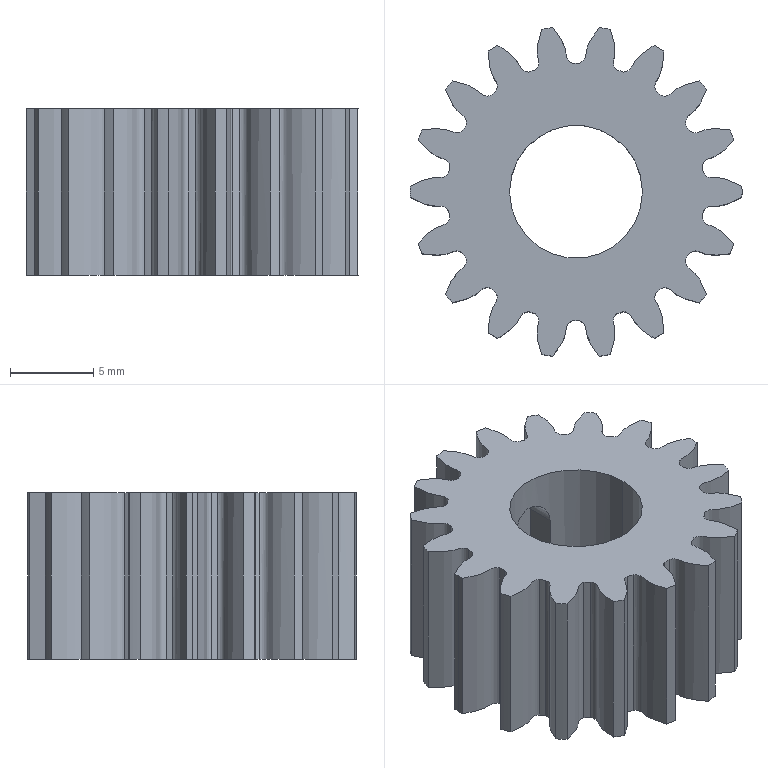Part | SolidWorks | features ICE 3, CirPattern 1, Extrusion 1, RefAxis 1 | 1 solid | 82 faces | box 20 x 19.803 x 10 mm | volume 1962 mm3 | cylinder 41 | spline 36 | plane 5 | commonest cylinder face diameters 20 x19 15.5 x18 3 x2 8 x2